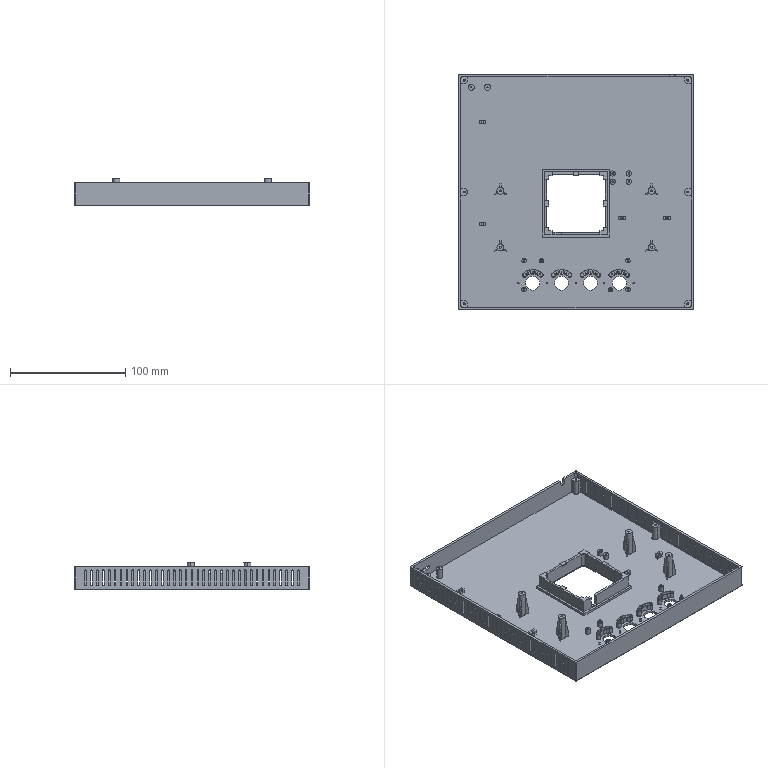Part | SolidWorks | features ICE 29, Fillet 5, Chamfer 3, Extrusion 1, MirrorPattern 1, Shell 1 | 1 solid | 884 faces | box 204 x 204 x 24 mm | volume 116811 mm3 | plane 495 | cylinder 381 | cone 4 | torus 4 | commonest cylinder face diameters 1.5 x164 0.8 x32 3 x24 4 x24 1.3 x22 17 x16